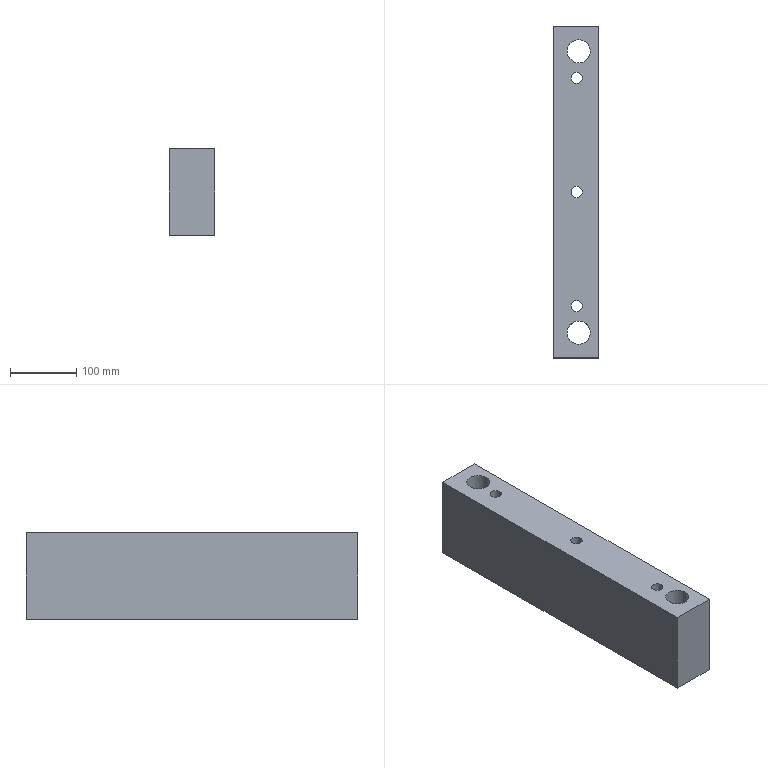Part | STEP file | SL2-MOLD_id746_xmt_txt | 1 solid | 11 faces | box 68 x 500 x 130 mm | volume 4081328 mm3 | plane 6 | cylinder 5 | commonest cylinder face diameters 17 x3 35 x2
STEP:
#1=CARTESIAN_POINT('',(-156.5,262.,-244.));
#2=VERTEX_POINT('',#1);
#3=CARTESIAN_POINT('',(-165.,262.,-244.));
#4=DIRECTION('',(0.,0.,1.));
#5=DIRECTION('',(1.,0.,0.));
#6=AXIS2_PLACEMENT_3D('',#3,#4,#5);
#7=CIRCLE('',#6,8.5);
#8=EDGE_CURVE('',#2,#2,#7,.T.);
#9=ORIENTED_EDGE('',*,*,#8,.T.);
#10=EDGE_LOOP('',(#9));
#11=FACE_BOUND('',#10,.T.);
#12=CARTESIAN_POINT('',(-156.5,90.,-244.));
#13=VERTEX_POINT('',#12);
#14=CARTESIAN_POINT('',(-165.,90.,-244.));
#15=DIRECTION('',(0.,0.,1.));
#16=DIRECTION('',(1.,0.,0.));
#17=AXIS2_PLACEMENT_3D('',#14,#15,#16);
#18=CIRCLE('',#17,8.5);
#19=EDGE_CURVE('',#13,#13,#18,.T.);
#20=ORIENTED_EDGE('',*,*,#19,.T.);
#21=EDGE_LOOP('',(#20));
#22=FACE_BOUND('',#21,.T.);
#23=CARTESIAN_POINT('',(-156.5,-82.,-244.));
#24=VERTEX_POINT('',#23);
#25=CARTESIAN_POINT('',(-165.,-82.,-244.));
#26=DIRECTION('',(0.,0.,1.));
#27=DIRECTION('',(1.,0.,0.));
#28=AXIS2_PLACEMENT_3D('',#25,#26,#27);
#29=CIRCLE('',#28,8.5);
#30=EDGE_CURVE('',#24,#24,#29,.T.);
#31=ORIENTED_EDGE('',*,*,#30,.T.);
#32=EDGE_LOOP('',(#31));
#33=FACE_BOUND('',#32,.T.);
#34=CARTESIAN_POINT('',(-144.5,-122.,-244.));
#35=VERTEX_POINT('',#34);
#36=CARTESIAN_POINT('',(-162.,-122.,-244.));
#37=DIRECTION('',(0.,0.,-1.));
#38=DIRECTION('',(1.,0.,0.));
#39=AXIS2_PLACEMENT_3D('',#36,#37,#38);
#40=CIRCLE('',#39,17.5);
#41=EDGE_CURVE('',#35,#35,#40,.T.);
#42=ORIENTED_EDGE('',*,*,#41,.F.);
#43=EDGE_LOOP('',(#42));
#44=FACE_BOUND('',#43,.T.);
#45=CARTESIAN_POINT('',(-132.,340.,-244.));
#46=VERTEX_POINT('',#45);
#47=CARTESIAN_POINT('',(-200.,340.,-244.));
#48=VERTEX_POINT('',#47);
#49=CARTESIAN_POINT('',(0.,340.,-244.));
#50=DIRECTION('',(-1.,0.,0.));
#51=VECTOR('',#50,1.);
#52=LINE('',#49,#51);
#53=EDGE_CURVE('',#46,#48,#52,.T.);
#54=ORIENTED_EDGE('',*,*,#53,.F.);
#55=CARTESIAN_POINT('',(-132.,-160.,-244.));
#56=VERTEX_POINT('',#55);
#57=CARTESIAN_POINT('',(-132.,0.,-244.));
#58=DIRECTION('',(0.,1.,0.));
#59=VECTOR('',#58,1.);
#60=LINE('',#57,#59);
#61=EDGE_CURVE('',#56,#46,#60,.T.);
#62=ORIENTED_EDGE('',*,*,#61,.F.);
#63=CARTESIAN_POINT('',(-200.,-160.,-244.));
#64=VERTEX_POINT('',#63);
#65=CARTESIAN_POINT('',(0.,-160.,-244.));
#66=DIRECTION('',(1.,0.,0.));
#67=VECTOR('',#66,1.);
#68=LINE('',#65,#67);
#69=EDGE_CURVE('',#64,#56,#68,.T.);
#70=ORIENTED_EDGE('',*,*,#69,.F.);
#71=CARTESIAN_POINT('',(-200.,0.,-244.));
#72=DIRECTION('',(0.,-1.,0.));
#73=VECTOR('',#72,1.);
#74=LINE('',#71,#73);
#75=EDGE_CURVE('',#48,#64,#74,.T.);
#76=ORIENTED_EDGE('',*,*,#75,.F.);
#77=EDGE_LOOP('',(#54,#62,#70,#76));
#78=FACE_BOUND('',#77,.T.);
#79=CARTESIAN_POINT('',(-144.5,302.,-244.));
#80=VERTEX_POINT('',#79);
#81=CARTESIAN_POINT('',(-162.,302.,-244.));
#82=DIRECTION('',(0.,0.,-1.));
#83=DIRECTION('',(1.,0.,0.));
#84=AXIS2_PLACEMENT_3D('',#81,#82,#83);
#85=CIRCLE('',#84,17.5);
#86=EDGE_CURVE('',#80,#80,#85,.T.);
#87=ORIENTED_EDGE('',*,*,#86,.F.);
#88=EDGE_LOOP('',(#87));
#89=FACE_BOUND('',#88,.T.);
#90=CARTESIAN_POINT('',(0.,0.,-244.));
#91=DIRECTION('',(0.,0.,1.));
#92=DIRECTION('',(1.,0.,0.));
#93=AXIS2_PLACEMENT_3D('',#90,#91,#92);
#94=PLANE('',#93);
#95=ADVANCED_FACE('',(#11,#22,#33,#44,#78,#89),#94,.F.);
#96=CARTESIAN_POINT('',(-200.,340.,-114.));
#97=VERTEX_POINT('',#96);
#98=CARTESIAN_POINT('',(-200.,-160.,-114.));
#99=VERTEX_POINT('',#98);
#100=CARTESIAN_POINT('',(-200.,0.,-114.));
#101=DIRECTION('',(0.,-1.,0.));
#102=VECTOR('',#101,1.);
#103=LINE('',#100,#102);
#104=EDGE_CURVE('',#97,#99,#103,.T.);
#105=ORIENTED_EDGE('',*,*,#104,.F.);
#106=CARTESIAN_POINT('',(-200.,340.,-244.));
#107=DIRECTION('',(0.,0.,1.));
#108=VECTOR('',#107,1.);
#109=LINE('',#106,#108);
#110=EDGE_CURVE('',#48,#97,#109,.T.);
#111=ORIENTED_EDGE('',*,*,#110,.F.);
#112=ORIENTED_EDGE('',*,*,#75,.T.);
#113=CARTESIAN_POINT('',(-200.,-160.,-244.));
#114=DIRECTION('',(0.,0.,1.));
#115=VECTOR('',#114,1.);
#116=LINE('',#113,#115);
#117=EDGE_CURVE('',#64,#99,#116,.T.);
#118=ORIENTED_EDGE('',*,*,#117,.T.);
#119=EDGE_LOOP('',(#105,#111,#112,#118));
#120=FACE_OUTER_BOUND('',#119,.T.);
#121=CARTESIAN_POINT('',(-200.,0.,-244.));
#122=DIRECTION('',(-1.,0.,0.));
#123=DIRECTION('',(0.,0.,1.));
#124=AXIS2_PLACEMENT_3D('',#121,#122,#123);
#125=PLANE('',#124);
#126=ADVANCED_FACE('',(#120),#125,.T.);
#127=CARTESIAN_POINT('',(-156.5,262.,-114.));
#128=VERTEX_POINT('',#127);
#129=CARTESIAN_POINT('',(-165.,262.,-114.));
#130=DIRECTION('',(0.,0.,1.));
#131=DIRECTION('',(1.,0.,0.));
#132=AXIS2_PLACEMENT_3D('',#129,#130,#131);
#133=CIRCLE('',#132,8.5);
#134=EDGE_CURVE('',#128,#128,#133,.T.);
#135=ORIENTED_EDGE('',*,*,#134,.F.);
#136=EDGE_LOOP('',(#135));
#137=FACE_BOUND('',#136,.T.);
#138=CARTESIAN_POINT('',(-156.5,90.,-114.));
#139=VERTEX_POINT('',#138);
#140=CARTESIAN_POINT('',(-165.,90.,-114.));
#141=DIRECTION('',(0.,0.,1.));
#142=DIRECTION('',(1.,0.,0.));
#143=AXIS2_PLACEMENT_3D('',#140,#141,#142);
#144=CIRCLE('',#143,8.5);
#145=EDGE_CURVE('',#139,#139,#144,.T.);
#146=ORIENTED_EDGE('',*,*,#145,.F.);
#147=EDGE_LOOP('',(#146));
#148=FACE_BOUND('',#147,.T.);
#149=CARTESIAN_POINT('',(-156.5,-82.,-114.));
#150=VERTEX_POINT('',#149);
#151=CARTESIAN_POINT('',(-165.,-82.,-114.));
#152=DIRECTION('',(0.,0.,1.));
#153=DIRECTION('',(1.,0.,0.));
#154=AXIS2_PLACEMENT_3D('',#151,#152,#153);
#155=CIRCLE('',#154,8.5);
#156=EDGE_CURVE('',#150,#150,#155,.T.);
#157=ORIENTED_EDGE('',*,*,#156,.F.);
#158=EDGE_LOOP('',(#157));
#159=FACE_BOUND('',#158,.T.);
#160=CARTESIAN_POINT('',(-144.5,-122.,-114.));
#161=VERTEX_POINT('',#160);
#162=CARTESIAN_POINT('',(-162.,-122.,-114.));
#163=DIRECTION('',(0.,0.,-1.));
#164=DIRECTION('',(1.,0.,0.));
#165=AXIS2_PLACEMENT_3D('',#162,#163,#164);
#166=CIRCLE('',#165,17.5);
#167=EDGE_CURVE('',#161,#161,#166,.T.);
#168=ORIENTED_EDGE('',*,*,#167,.T.);
#169=EDGE_LOOP('',(#168));
#170=FACE_BOUND('',#169,.T.);
#171=CARTESIAN_POINT('',(-144.5,302.,-114.));
#172=VERTEX_POINT('',#171);
#173=CARTESIAN_POINT('',(-162.,302.,-114.));
#174=DIRECTION('',(0.,0.,-1.));
#175=DIRECTION('',(1.,0.,0.));
#176=AXIS2_PLACEMENT_3D('',#173,#174,#175);
#177=CIRCLE('',#176,17.5);
#178=EDGE_CURVE('',#172,#172,#177,.T.);
#179=ORIENTED_EDGE('',*,*,#178,.T.);
#180=EDGE_LOOP('',(#179));
#181=FACE_BOUND('',#180,.T.);
#182=CARTESIAN_POINT('',(-132.,-160.,-114.));
#183=VERTEX_POINT('',#182);
#184=CARTESIAN_POINT('',(-132.,340.,-114.));
#185=VERTEX_POINT('',#184);
#186=CARTESIAN_POINT('',(-132.,0.,-114.));
#187=DIRECTION('',(0.,1.,0.));
#188=VECTOR('',#187,1.);
#189=LINE('',#186,#188);
#190=EDGE_CURVE('',#183,#185,#189,.T.);
#191=ORIENTED_EDGE('',*,*,#190,.T.);
#192=CARTESIAN_POINT('',(0.,340.,-114.));
#193=DIRECTION('',(-1.,0.,0.));
#194=VECTOR('',#193,1.);
#195=LINE('',#192,#194);
#196=EDGE_CURVE('',#185,#97,#195,.T.);
#197=ORIENTED_EDGE('',*,*,#196,.T.);
#198=ORIENTED_EDGE('',*,*,#104,.T.);
#199=CARTESIAN_POINT('',(0.,-160.,-114.));
#200=DIRECTION('',(1.,0.,0.));
#201=VECTOR('',#200,1.);
#202=LINE('',#199,#201);
#203=EDGE_CURVE('',#99,#183,#202,.T.);
#204=ORIENTED_EDGE('',*,*,#203,.T.);
#205=EDGE_LOOP('',(#191,#197,#198,#204));
#206=FACE_BOUND('',#205,.T.);
#207=CARTESIAN_POINT('',(0.,0.,-114.));
#208=DIRECTION('',(0.,0.,1.));
#209=DIRECTION('',(1.,0.,0.));
#210=AXIS2_PLACEMENT_3D('',#207,#208,#209);
#211=PLANE('',#210);
#212=ADVANCED_FACE('',(#137,#148,#159,#170,#181,#206),#211,.T.);
#213=CARTESIAN_POINT('',(-132.,340.,-244.));
#214=DIRECTION('',(0.,0.,-1.));
#215=VECTOR('',#214,1.);
#216=LINE('',#213,#215);
#217=EDGE_CURVE('',#185,#46,#216,.T.);
#218=ORIENTED_EDGE('',*,*,#217,.T.);
#219=ORIENTED_EDGE('',*,*,#53,.T.);
#220=ORIENTED_EDGE('',*,*,#110,.T.);
#221=ORIENTED_EDGE('',*,*,#196,.F.);
#222=EDGE_LOOP('',(#218,#219,#220,#221));
#223=FACE_OUTER_BOUND('',#222,.T.);
#224=CARTESIAN_POINT('',(0.,340.,-244.));
#225=DIRECTION('',(0.,1.,0.));
#226=DIRECTION('',(0.,0.,1.));
#227=AXIS2_PLACEMENT_3D('',#224,#225,#226);
#228=PLANE('',#227);
#229=ADVANCED_FACE('',(#223),#228,.T.);
#230=CARTESIAN_POINT('',(-132.,-160.,-244.));
#231=DIRECTION('',(0.,0.,1.));
#232=VECTOR('',#231,1.);
#233=LINE('',#230,#232);
#234=EDGE_CURVE('',#56,#183,#233,.T.);
#235=ORIENTED_EDGE('',*,*,#234,.T.);
#236=ORIENTED_EDGE('',*,*,#203,.F.);
#237=ORIENTED_EDGE('',*,*,#117,.F.);
#238=ORIENTED_EDGE('',*,*,#69,.T.);
#239=EDGE_LOOP('',(#235,#236,#237,#238));
#240=FACE_OUTER_BOUND('',#239,.T.);
#241=CARTESIAN_POINT('',(0.,-160.,-244.));
#242=DIRECTION('',(0.,-1.,0.));
#243=DIRECTION('',(0.,0.,-1.));
#244=AXIS2_PLACEMENT_3D('',#241,#242,#243);
#245=PLANE('',#244);
#246=ADVANCED_FACE('',(#240),#245,.T.);
#247=ORIENTED_EDGE('',*,*,#217,.F.);
#248=ORIENTED_EDGE('',*,*,#190,.F.);
#249=ORIENTED_EDGE('',*,*,#234,.F.);
#250=ORIENTED_EDGE('',*,*,#61,.T.);
#251=EDGE_LOOP('',(#247,#248,#249,#250));
#252=FACE_OUTER_BOUND('',#251,.T.);
#253=CARTESIAN_POINT('',(-132.,90.,-179.));
#254=DIRECTION('',(-1.,0.,0.));
#255=DIRECTION('',(0.,0.,1.));
#256=AXIS2_PLACEMENT_3D('',#253,#254,#255);
#257=PLANE('',#256);
#258=ADVANCED_FACE('',(#252),#257,.F.);
#259=ORIENTED_EDGE('',*,*,#178,.F.);
#260=EDGE_LOOP('',(#259));
#261=FACE_BOUND('',#260,.T.);
#262=ORIENTED_EDGE('',*,*,#86,.T.);
#263=EDGE_LOOP('',(#262));
#264=FACE_BOUND('',#263,.T.);
#265=CARTESIAN_POINT('',(-162.,302.,3221.8));
#266=DIRECTION('',(0.,0.,-1.));
#267=DIRECTION('',(-1.,0.,0.));
#268=AXIS2_PLACEMENT_3D('',#265,#266,#267);
#269=CYLINDRICAL_SURFACE('',#268,17.5);
#270=ADVANCED_FACE('',(#261,#264),#269,.F.);
#271=ORIENTED_EDGE('',*,*,#167,.F.);
#272=EDGE_LOOP('',(#271));
#273=FACE_BOUND('',#272,.T.);
#274=ORIENTED_EDGE('',*,*,#41,.T.);
#275=EDGE_LOOP('',(#274));
#276=FACE_BOUND('',#275,.T.);
#277=CARTESIAN_POINT('',(-162.,-122.,3221.8));
#278=DIRECTION('',(0.,0.,-1.));
#279=DIRECTION('',(-1.,0.,0.));
#280=AXIS2_PLACEMENT_3D('',#277,#278,#279);
#281=CYLINDRICAL_SURFACE('',#280,17.5);
#282=ADVANCED_FACE('',(#273,#276),#281,.F.);
#283=ORIENTED_EDGE('',*,*,#156,.T.);
#284=EDGE_LOOP('',(#283));
#285=FACE_BOUND('',#284,.T.);
#286=ORIENTED_EDGE('',*,*,#30,.F.);
#287=EDGE_LOOP('',(#286));
#288=FACE_BOUND('',#287,.T.);
#289=CARTESIAN_POINT('',(-165.,-82.,-2215.55));
#290=DIRECTION('',(0.,0.,1.));
#291=DIRECTION('',(1.,0.,0.));
#292=AXIS2_PLACEMENT_3D('',#289,#290,#291);
#293=CYLINDRICAL_SURFACE('',#292,8.5);
#294=ADVANCED_FACE('',(#285,#288),#293,.F.);
#295=ORIENTED_EDGE('',*,*,#145,.T.);
#296=EDGE_LOOP('',(#295));
#297=FACE_BOUND('',#296,.T.);
#298=ORIENTED_EDGE('',*,*,#19,.F.);
#299=EDGE_LOOP('',(#298));
#300=FACE_BOUND('',#299,.T.);
#301=CARTESIAN_POINT('',(-165.,90.,-2215.55));
#302=DIRECTION('',(0.,0.,1.));
#303=DIRECTION('',(1.,0.,0.));
#304=AXIS2_PLACEMENT_3D('',#301,#302,#303);
#305=CYLINDRICAL_SURFACE('',#304,8.5);
#306=ADVANCED_FACE('',(#297,#300),#305,.F.);
#307=ORIENTED_EDGE('',*,*,#134,.T.);
#308=EDGE_LOOP('',(#307));
#309=FACE_BOUND('',#308,.T.);
#310=ORIENTED_EDGE('',*,*,#8,.F.);
#311=EDGE_LOOP('',(#310));
#312=FACE_BOUND('',#311,.T.);
#313=CARTESIAN_POINT('',(-165.,262.,-2215.55));
#314=DIRECTION('',(0.,0.,1.));
#315=DIRECTION('',(1.,0.,0.));
#316=AXIS2_PLACEMENT_3D('',#313,#314,#315);
#317=CYLINDRICAL_SURFACE('',#316,8.5);
#318=ADVANCED_FACE('',(#309,#312),#317,.F.);
#319=CLOSED_SHELL('',(#95,#126,#212,#229,#246,#258,#270,#282,#294,#306,#318));
#320=MANIFOLD_SOLID_BREP('',#319);
#321=(LENGTH_UNIT()NAMED_UNIT(*)SI_UNIT(.MILLI.,.METRE.));
#322=UNCERTAINTY_MEASURE_WITH_UNIT(LENGTH_MEASURE(0.00002),#321,'','');
#323=(NAMED_UNIT(*)PLANE_ANGLE_UNIT()SI_UNIT($,.RADIAN.));
#324=PLANE_ANGLE_MEASURE_WITH_UNIT(PLANE_ANGLE_MEASURE(0.01745),#323);
#325=DIMENSIONAL_EXPONENTS(0.,0.,0.,0.,0.,0.,0.);
#326=(CONVERSION_BASED_UNIT('DEGREE',#324)NAMED_UNIT(#325)PLANE_ANGLE_UNIT());
#327=(NAMED_UNIT(*)SI_UNIT($,.STERADIAN.)SOLID_ANGLE_UNIT());
#328=(GEOMETRIC_REPRESENTATION_CONTEXT(3)GLOBAL_UNCERTAINTY_ASSIGNED_CONTEXT((#322))GLOBAL_UNIT_ASSIGNED_CONTEXT((#321,#326,#327))REPRESENTATION_CONTEXT('',''));
#329=ADVANCED_BREP_SHAPE_REPRESENTATION('',(#320),#328);